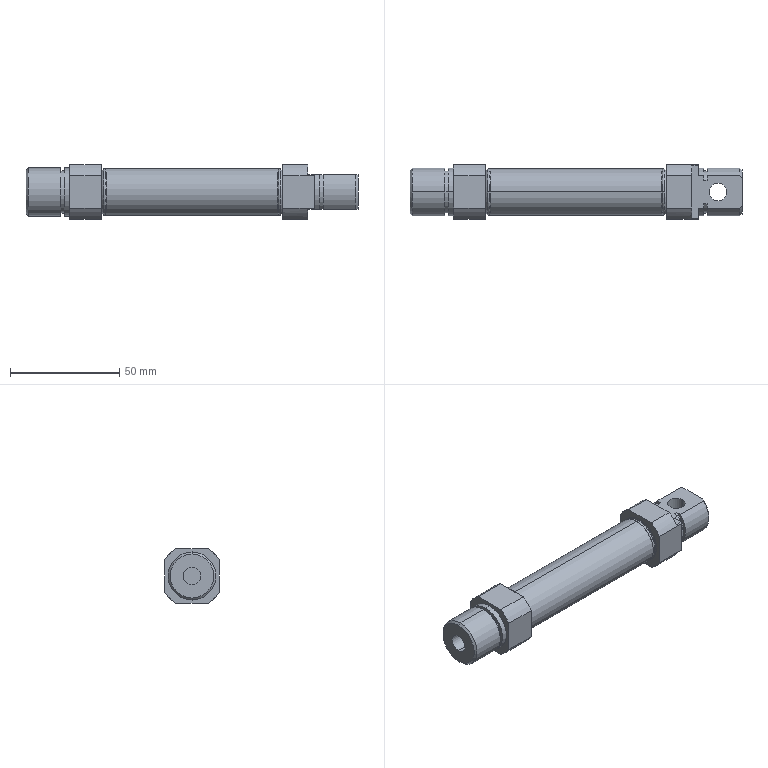Part | SolidWorks | features BaseBody 1 | 1 solid | 88 faces | box 152 x 25 x 25 mm | volume 36609 mm3 | cylinder 36 | plane 32 | cone 16 | torus 4 | commonest cylinder face diameters 22 x8 29 x8 21.4 x6 8 x4 8.566 x4 19.25 x4